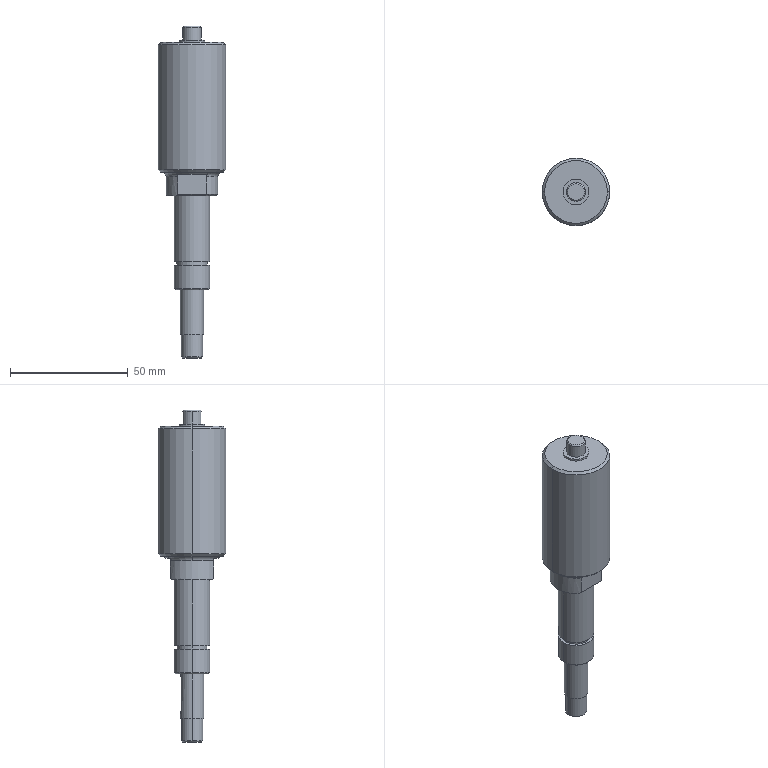Part | STEP file | 10000020465swp000-1 | 1 solid | 59 faces | box 28.65 x 28.65 x 140.9 mm | volume 48218 mm3 | cylinder 24 | plane 19 | cone 14 | torus 2 | commonest cylinder face diameters 15 x4 4 x3 22 x3 3.3 x2 8 x2 9 x2